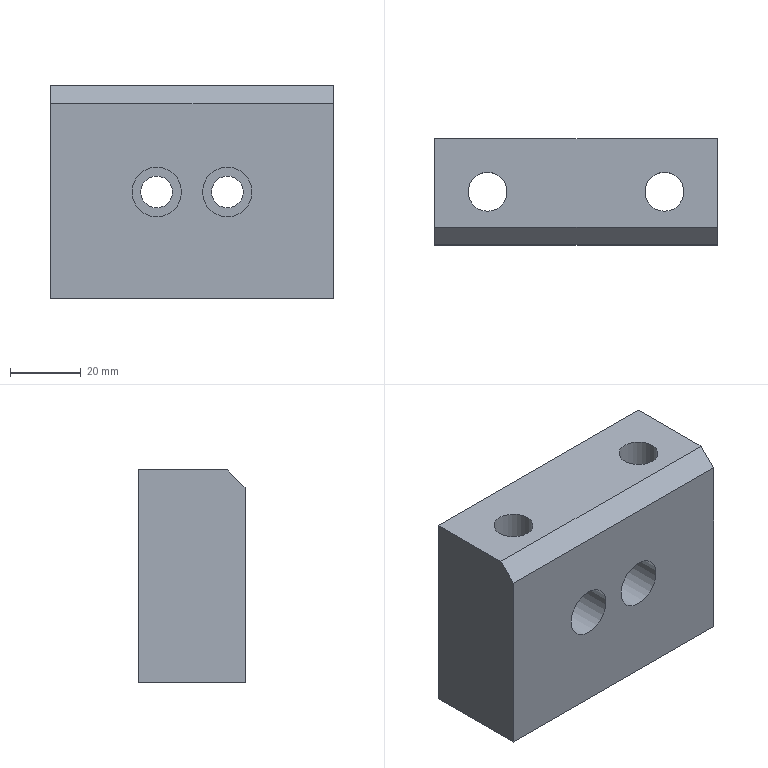Part | NX | features solid 2 | 1 solid | 19 faces | box 80 x 30 x 60 mm | volume 114333 mm3 | plane 11 | cylinder 8 | commonest cylinder face diameters 9 x2 11 x2 14 x2 17.5 x2
STEP:
#1=CARTESIAN_POINT('',(-375.,504.,180.));
#2=VERTEX_POINT('',#1);
#3=CARTESIAN_POINT('',(-375.,529.,180.));
#4=VERTEX_POINT('',#3);
#5=CARTESIAN_POINT('',(-375.,499.,180.));
#6=DIRECTION('',(0.,1.,0.));
#7=VECTOR('',#6,1000.);
#8=LINE('',#5,#7);
#9=EDGE_CURVE('',#2,#4,#8,.T.);
#10=ORIENTED_EDGE('',*,*,#9,.F.);
#11=CARTESIAN_POINT('',(-295.,504.,180.));
#12=VERTEX_POINT('',#11);
#13=CARTESIAN_POINT('',(-325.,504.,180.));
#14=DIRECTION('',(1.,0.,0.));
#15=VECTOR('',#14,1000.);
#16=LINE('',#13,#15);
#17=EDGE_CURVE('',#2,#12,#16,.T.);
#18=ORIENTED_EDGE('',*,*,#17,.T.);
#19=CARTESIAN_POINT('',(-295.,529.,180.));
#20=VERTEX_POINT('',#19);
#21=CARTESIAN_POINT('',(-295.,519.,180.));
#22=DIRECTION('',(0.,1.,0.));
#23=VECTOR('',#22,1000.);
#24=LINE('',#21,#23);
#25=EDGE_CURVE('',#12,#20,#24,.T.);
#26=ORIENTED_EDGE('',*,*,#25,.T.);
#27=CARTESIAN_POINT('',(-325.,529.,180.));
#28=DIRECTION('',(-1.,0.,0.));
#29=VECTOR('',#28,1000.);
#30=LINE('',#27,#29);
#31=EDGE_CURVE('',#20,#4,#30,.T.);
#32=ORIENTED_EDGE('',*,*,#31,.T.);
#33=EDGE_LOOP('',(#10,#18,#26,#32));
#34=FACE_BOUND('',#33,.T.);
#35=CARTESIAN_POINT('',(-310.,519.5,180.));
#36=VERTEX_POINT('',#35);
#37=CARTESIAN_POINT('',(-310.,514.,180.));
#38=DIRECTION('',(0.,0.,-1.));
#39=DIRECTION('',(0.,1.,0.));
#40=AXIS2_PLACEMENT_3D('',#37,#38,#39);
#41=CIRCLE('',#40,5.5);
#42=EDGE_CURVE('',#36,#36,#41,.T.);
#43=ORIENTED_EDGE('',*,*,#42,.T.);
#44=EDGE_LOOP('',(#43));
#45=FACE_BOUND('',#44,.T.);
#46=CARTESIAN_POINT('',(-360.,519.5,180.));
#47=VERTEX_POINT('',#46);
#48=CARTESIAN_POINT('',(-360.,514.,180.));
#49=DIRECTION('',(0.,0.,-1.));
#50=DIRECTION('',(0.,1.,0.));
#51=AXIS2_PLACEMENT_3D('',#48,#49,#50);
#52=CIRCLE('',#51,5.5);
#53=EDGE_CURVE('',#47,#47,#52,.T.);
#54=ORIENTED_EDGE('',*,*,#53,.T.);
#55=EDGE_LOOP('',(#54));
#56=FACE_BOUND('',#55,.T.);
#57=CARTESIAN_POINT('',(-325.,519.,180.));
#58=DIRECTION('',(0.,0.,1.));
#59=DIRECTION('',(-1.,0.,0.));
#60=AXIS2_PLACEMENT_3D('',#57,#58,#59);
#61=PLANE('',#60);
#62=ADVANCED_FACE('',(#34,#45,#56),#61,.T.);
#63=CARTESIAN_POINT('',(-295.,499.,175.));
#64=VERTEX_POINT('',#63);
#65=CARTESIAN_POINT('',(-295.,501.5,177.5));
#66=DIRECTION('',(0.,0.7071,0.7071));
#67=VECTOR('',#66,1000.);
#68=LINE('',#65,#67);
#69=EDGE_CURVE('',#64,#12,#68,.T.);
#70=ORIENTED_EDGE('',*,*,#69,.F.);
#71=CARTESIAN_POINT('',(-295.,499.,120.));
#72=VERTEX_POINT('',#71);
#73=CARTESIAN_POINT('',(-295.,499.,175.));
#74=DIRECTION('',(0.,0.,1.));
#75=VECTOR('',#74,1000.);
#76=LINE('',#73,#75);
#77=EDGE_CURVE('',#64,#72,#76,.F.);
#78=ORIENTED_EDGE('',*,*,#77,.T.);
#79=CARTESIAN_POINT('',(-295.,529.,120.));
#80=VERTEX_POINT('',#79);
#81=CARTESIAN_POINT('',(-295.,662.,120.));
#82=DIRECTION('',(0.,-1.,0.));
#83=VECTOR('',#82,1000.);
#84=LINE('',#81,#83);
#85=EDGE_CURVE('',#72,#80,#84,.F.);
#86=ORIENTED_EDGE('',*,*,#85,.T.);
#87=CARTESIAN_POINT('',(-295.,529.,130.));
#88=DIRECTION('',(0.,0.,1.));
#89=VECTOR('',#88,1000.);
#90=LINE('',#87,#89);
#91=EDGE_CURVE('',#80,#20,#90,.T.);
#92=ORIENTED_EDGE('',*,*,#91,.T.);
#93=ORIENTED_EDGE('',*,*,#25,.F.);
#94=EDGE_LOOP('',(#70,#78,#86,#92,#93));
#95=FACE_BOUND('',#94,.T.);
#96=CARTESIAN_POINT('',(-295.,519.,130.));
#97=DIRECTION('',(1.,0.,0.));
#98=DIRECTION('',(0.,0.,1.));
#99=AXIS2_PLACEMENT_3D('',#96,#97,#98);
#100=PLANE('',#99);
#101=ADVANCED_FACE('',(#95),#100,.T.);
#102=CARTESIAN_POINT('',(-345.,529.,154.5));
#103=VERTEX_POINT('',#102);
#104=CARTESIAN_POINT('',(-345.,529.,150.));
#105=DIRECTION('',(0.,1.,0.));
#106=DIRECTION('',(0.,0.,1.));
#107=AXIS2_PLACEMENT_3D('',#104,#105,#106);
#108=CIRCLE('',#107,4.5);
#109=EDGE_CURVE('',#103,#103,#108,.T.);
#110=ORIENTED_EDGE('',*,*,#109,.F.);
#111=EDGE_LOOP('',(#110));
#112=FACE_BOUND('',#111,.T.);
#113=CARTESIAN_POINT('',(-325.,529.,154.5));
#114=VERTEX_POINT('',#113);
#115=CARTESIAN_POINT('',(-325.,529.,150.));
#116=DIRECTION('',(0.,1.,0.));
#117=DIRECTION('',(0.,0.,1.));
#118=AXIS2_PLACEMENT_3D('',#115,#116,#117);
#119=CIRCLE('',#118,4.5);
#120=EDGE_CURVE('',#114,#114,#119,.T.);
#121=ORIENTED_EDGE('',*,*,#120,.F.);
#122=EDGE_LOOP('',(#121));
#123=FACE_BOUND('',#122,.T.);
#124=CARTESIAN_POINT('',(-375.,529.,120.));
#125=VERTEX_POINT('',#124);
#126=CARTESIAN_POINT('',(-289.,529.,120.));
#127=DIRECTION('',(-1.,0.,0.));
#128=VECTOR('',#127,1000.);
#129=LINE('',#126,#128);
#130=EDGE_CURVE('',#125,#80,#129,.F.);
#131=ORIENTED_EDGE('',*,*,#130,.F.);
#132=CARTESIAN_POINT('',(-375.,529.,175.));
#133=DIRECTION('',(0.,0.,-1.));
#134=VECTOR('',#133,1000.);
#135=LINE('',#132,#134);
#136=EDGE_CURVE('',#4,#125,#135,.T.);
#137=ORIENTED_EDGE('',*,*,#136,.F.);
#138=ORIENTED_EDGE('',*,*,#31,.F.);
#139=ORIENTED_EDGE('',*,*,#91,.F.);
#140=EDGE_LOOP('',(#131,#137,#138,#139));
#141=FACE_BOUND('',#140,.T.);
#142=CARTESIAN_POINT('',(-335.,529.,175.));
#143=DIRECTION('',(0.,-1.,0.));
#144=DIRECTION('',(0.,0.,-1.));
#145=AXIS2_PLACEMENT_3D('',#142,#143,#144);
#146=PLANE('',#145);
#147=ADVANCED_FACE('',(#112,#123,#141),#146,.F.);
#148=CARTESIAN_POINT('',(-345.,499.,143.));
#149=VERTEX_POINT('',#148);
#150=CARTESIAN_POINT('',(-345.,499.,150.));
#151=DIRECTION('',(0.,-1.,0.));
#152=DIRECTION('',(0.,0.,-1.));
#153=AXIS2_PLACEMENT_3D('',#150,#151,#152);
#154=CIRCLE('',#153,7.);
#155=EDGE_CURVE('',#149,#149,#154,.T.);
#156=ORIENTED_EDGE('',*,*,#155,.F.);
#157=EDGE_LOOP('',(#156));
#158=FACE_BOUND('',#157,.T.);
#159=CARTESIAN_POINT('',(-375.,499.,175.));
#160=VERTEX_POINT('',#159);
#161=CARTESIAN_POINT('',(-375.,499.,120.));
#162=VERTEX_POINT('',#161);
#163=CARTESIAN_POINT('',(-375.,499.,175.));
#164=DIRECTION('',(0.,0.,1.));
#165=VECTOR('',#164,1000.);
#166=LINE('',#163,#165);
#167=EDGE_CURVE('',#160,#162,#166,.F.);
#168=ORIENTED_EDGE('',*,*,#167,.T.);
#169=CARTESIAN_POINT('',(-335.,499.,120.));
#170=DIRECTION('',(1.,0.,0.));
#171=VECTOR('',#170,1000.);
#172=LINE('',#169,#171);
#173=EDGE_CURVE('',#162,#72,#172,.T.);
#174=ORIENTED_EDGE('',*,*,#173,.T.);
#175=ORIENTED_EDGE('',*,*,#77,.F.);
#176=CARTESIAN_POINT('',(-335.,499.,175.));
#177=DIRECTION('',(-1.,0.,0.));
#178=VECTOR('',#177,1000.);
#179=LINE('',#176,#178);
#180=EDGE_CURVE('',#160,#64,#179,.F.);
#181=ORIENTED_EDGE('',*,*,#180,.F.);
#182=EDGE_LOOP('',(#168,#174,#175,#181));
#183=FACE_BOUND('',#182,.T.);
#184=CARTESIAN_POINT('',(-325.,499.,143.));
#185=VERTEX_POINT('',#184);
#186=CARTESIAN_POINT('',(-325.,499.,150.));
#187=DIRECTION('',(0.,-1.,0.));
#188=DIRECTION('',(0.,0.,-1.));
#189=AXIS2_PLACEMENT_3D('',#186,#187,#188);
#190=CIRCLE('',#189,7.);
#191=EDGE_CURVE('',#185,#185,#190,.T.);
#192=ORIENTED_EDGE('',*,*,#191,.F.);
#193=EDGE_LOOP('',(#192));
#194=FACE_BOUND('',#193,.T.);
#195=CARTESIAN_POINT('',(-335.,499.,175.));
#196=DIRECTION('',(0.,-1.,0.));
#197=DIRECTION('',(0.,0.,-1.));
#198=AXIS2_PLACEMENT_3D('',#195,#196,#197);
#199=PLANE('',#198);
#200=ADVANCED_FACE('',(#158,#183,#194),#199,.T.);
#201=CARTESIAN_POINT('',(-360.,522.75,120.));
#202=VERTEX_POINT('',#201);
#203=CARTESIAN_POINT('',(-360.,514.,120.));
#204=DIRECTION('',(0.,0.,-1.));
#205=DIRECTION('',(0.,1.,0.));
#206=AXIS2_PLACEMENT_3D('',#203,#204,#205);
#207=CIRCLE('',#206,8.75);
#208=EDGE_CURVE('',#202,#202,#207,.F.);
#209=ORIENTED_EDGE('',*,*,#208,.T.);
#210=EDGE_LOOP('',(#209));
#211=FACE_BOUND('',#210,.T.);
#212=CARTESIAN_POINT('',(-310.,522.75,120.));
#213=VERTEX_POINT('',#212);
#214=CARTESIAN_POINT('',(-310.,514.,120.));
#215=DIRECTION('',(0.,0.,-1.));
#216=DIRECTION('',(0.,1.,0.));
#217=AXIS2_PLACEMENT_3D('',#214,#215,#216);
#218=CIRCLE('',#217,8.75);
#219=EDGE_CURVE('',#213,#213,#218,.F.);
#220=ORIENTED_EDGE('',*,*,#219,.T.);
#221=EDGE_LOOP('',(#220));
#222=FACE_BOUND('',#221,.T.);
#223=CARTESIAN_POINT('',(-375.,662.,120.));
#224=DIRECTION('',(0.,-1.,0.));
#225=VECTOR('',#224,1000.);
#226=LINE('',#223,#225);
#227=EDGE_CURVE('',#162,#125,#226,.F.);
#228=ORIENTED_EDGE('',*,*,#227,.T.);
#229=ORIENTED_EDGE('',*,*,#130,.T.);
#230=ORIENTED_EDGE('',*,*,#85,.F.);
#231=ORIENTED_EDGE('',*,*,#173,.F.);
#232=EDGE_LOOP('',(#228,#229,#230,#231));
#233=FACE_BOUND('',#232,.T.);
#234=CARTESIAN_POINT('',(-289.,662.,120.));
#235=DIRECTION('',(0.,0.,-1.));
#236=DIRECTION('',(1.,0.,0.));
#237=AXIS2_PLACEMENT_3D('',#234,#235,#236);
#238=PLANE('',#237);
#239=ADVANCED_FACE('',(#211,#222,#233),#238,.T.);
#240=ORIENTED_EDGE('',*,*,#9,.T.);
#241=ORIENTED_EDGE('',*,*,#136,.T.);
#242=ORIENTED_EDGE('',*,*,#227,.F.);
#243=ORIENTED_EDGE('',*,*,#167,.F.);
#244=CARTESIAN_POINT('',(-375.,499.,175.));
#245=DIRECTION('',(0.,-0.7071,-0.7071));
#246=VECTOR('',#245,1000.);
#247=LINE('',#244,#246);
#248=EDGE_CURVE('',#2,#160,#247,.T.);
#249=ORIENTED_EDGE('',*,*,#248,.F.);
#250=EDGE_LOOP('',(#240,#241,#242,#243,#249));
#251=FACE_BOUND('',#250,.T.);
#252=CARTESIAN_POINT('',(-375.,499.,175.));
#253=DIRECTION('',(1.,0.,0.));
#254=DIRECTION('',(0.,-0.6428,0.766));
#255=AXIS2_PLACEMENT_3D('',#252,#253,#254);
#256=PLANE('',#255);
#257=ADVANCED_FACE('',(#251),#256,.F.);
#258=CARTESIAN_POINT('',(-310.,508.5,160.));
#259=VERTEX_POINT('',#258);
#260=CARTESIAN_POINT('',(-310.,514.,160.));
#261=DIRECTION('',(0.,0.,1.));
#262=DIRECTION('',(0.,-1.,0.));
#263=AXIS2_PLACEMENT_3D('',#260,#261,#262);
#264=CIRCLE('',#263,5.5);
#265=EDGE_CURVE('',#259,#259,#264,.T.);
#266=ORIENTED_EDGE('',*,*,#265,.F.);
#267=EDGE_LOOP('',(#266));
#268=FACE_BOUND('',#267,.T.);
#269=ORIENTED_EDGE('',*,*,#42,.F.);
#270=EDGE_LOOP('',(#269));
#271=FACE_BOUND('',#270,.T.);
#272=CARTESIAN_POINT('',(-310.,514.,205.));
#273=DIRECTION('',(0.,0.,1.));
#274=DIRECTION('',(0.,-1.,0.));
#275=AXIS2_PLACEMENT_3D('',#272,#273,#274);
#276=CYLINDRICAL_SURFACE('',#275,5.5);
#277=ADVANCED_FACE('',(#268,#271),#276,.F.);
#278=ORIENTED_EDGE('',*,*,#265,.T.);
#279=EDGE_LOOP('',(#278));
#280=FACE_BOUND('',#279,.T.);
#281=CARTESIAN_POINT('',(-310.,505.25,160.));
#282=VERTEX_POINT('',#281);
#283=CARTESIAN_POINT('',(-310.,514.,160.));
#284=DIRECTION('',(0.,0.,1.));
#285=DIRECTION('',(0.,-1.,0.));
#286=AXIS2_PLACEMENT_3D('',#283,#284,#285);
#287=CIRCLE('',#286,8.75);
#288=EDGE_CURVE('',#282,#282,#287,.T.);
#289=ORIENTED_EDGE('',*,*,#288,.F.);
#290=EDGE_LOOP('',(#289));
#291=FACE_BOUND('',#290,.T.);
#292=CARTESIAN_POINT('',(-310.,514.,160.));
#293=DIRECTION('',(0.,0.,1.));
#294=DIRECTION('',(0.,-1.,0.));
#295=AXIS2_PLACEMENT_3D('',#292,#293,#294);
#296=PLANE('',#295);
#297=ADVANCED_FACE('',(#280,#291),#296,.F.);
#298=ORIENTED_EDGE('',*,*,#288,.T.);
#299=EDGE_LOOP('',(#298));
#300=FACE_BOUND('',#299,.T.);
#301=ORIENTED_EDGE('',*,*,#219,.F.);
#302=EDGE_LOOP('',(#301));
#303=FACE_BOUND('',#302,.T.);
#304=CARTESIAN_POINT('',(-310.,514.,125.));
#305=DIRECTION('',(0.,0.,1.));
#306=DIRECTION('',(0.,-1.,0.));
#307=AXIS2_PLACEMENT_3D('',#304,#305,#306);
#308=CYLINDRICAL_SURFACE('',#307,8.75);
#309=ADVANCED_FACE('',(#300,#303),#308,.F.);
#310=CARTESIAN_POINT('',(-325.,509.,154.5));
#311=VERTEX_POINT('',#310);
#312=CARTESIAN_POINT('',(-325.,509.,150.));
#313=DIRECTION('',(0.,1.,0.));
#314=DIRECTION('',(0.,0.,1.));
#315=AXIS2_PLACEMENT_3D('',#312,#313,#314);
#316=CIRCLE('',#315,4.5);
#317=EDGE_CURVE('',#311,#311,#316,.T.);
#318=ORIENTED_EDGE('',*,*,#317,.F.);
#319=EDGE_LOOP('',(#318));
#320=FACE_BOUND('',#319,.T.);
#321=ORIENTED_EDGE('',*,*,#120,.T.);
#322=EDGE_LOOP('',(#321));
#323=FACE_BOUND('',#322,.T.);
#324=CARTESIAN_POINT('',(-325.,529.,150.));
#325=DIRECTION('',(0.,-1.,0.));
#326=DIRECTION('',(0.,0.,-1.));
#327=AXIS2_PLACEMENT_3D('',#324,#325,#326);
#328=CYLINDRICAL_SURFACE('',#327,4.5);
#329=ADVANCED_FACE('',(#320,#323),#328,.F.);
#330=CARTESIAN_POINT('',(-345.,509.,154.5));
#331=VERTEX_POINT('',#330);
#332=CARTESIAN_POINT('',(-345.,509.,150.));
#333=DIRECTION('',(0.,1.,0.));
#334=DIRECTION('',(0.,0.,1.));
#335=AXIS2_PLACEMENT_3D('',#332,#333,#334);
#336=CIRCLE('',#335,4.5);
#337=EDGE_CURVE('',#331,#331,#336,.T.);
#338=ORIENTED_EDGE('',*,*,#337,.F.);
#339=EDGE_LOOP('',(#338));
#340=FACE_BOUND('',#339,.T.);
#341=ORIENTED_EDGE('',*,*,#109,.T.);
#342=EDGE_LOOP('',(#341));
#343=FACE_BOUND('',#342,.T.);
#344=CARTESIAN_POINT('',(-345.,529.,150.));
#345=DIRECTION('',(0.,-1.,0.));
#346=DIRECTION('',(0.,0.,-1.));
#347=AXIS2_PLACEMENT_3D('',#344,#345,#346);
#348=CYLINDRICAL_SURFACE('',#347,4.5);
#349=ADVANCED_FACE('',(#340,#343),#348,.F.);
#350=CARTESIAN_POINT('',(-360.,508.5,160.));
#351=VERTEX_POINT('',#350);
#352=CARTESIAN_POINT('',(-360.,514.,160.));
#353=DIRECTION('',(0.,0.,1.));
#354=DIRECTION('',(0.,-1.,0.));
#355=AXIS2_PLACEMENT_3D('',#352,#353,#354);
#356=CIRCLE('',#355,5.5);
#357=EDGE_CURVE('',#351,#351,#356,.T.);
#358=ORIENTED_EDGE('',*,*,#357,.F.);
#359=EDGE_LOOP('',(#358));
#360=FACE_BOUND('',#359,.T.);
#361=ORIENTED_EDGE('',*,*,#53,.F.);
#362=EDGE_LOOP('',(#361));
#363=FACE_BOUND('',#362,.T.);
#364=CARTESIAN_POINT('',(-360.,514.,205.));
#365=DIRECTION('',(0.,0.,1.));
#366=DIRECTION('',(0.,-1.,0.));
#367=AXIS2_PLACEMENT_3D('',#364,#365,#366);
#368=CYLINDRICAL_SURFACE('',#367,5.5);
#369=ADVANCED_FACE('',(#360,#363),#368,.F.);
#370=ORIENTED_EDGE('',*,*,#357,.T.);
#371=EDGE_LOOP('',(#370));
#372=FACE_BOUND('',#371,.T.);
#373=CARTESIAN_POINT('',(-360.,505.25,160.));
#374=VERTEX_POINT('',#373);
#375=CARTESIAN_POINT('',(-360.,514.,160.));
#376=DIRECTION('',(0.,0.,1.));
#377=DIRECTION('',(0.,-1.,0.));
#378=AXIS2_PLACEMENT_3D('',#375,#376,#377);
#379=CIRCLE('',#378,8.75);
#380=EDGE_CURVE('',#374,#374,#379,.T.);
#381=ORIENTED_EDGE('',*,*,#380,.F.);
#382=EDGE_LOOP('',(#381));
#383=FACE_BOUND('',#382,.T.);
#384=CARTESIAN_POINT('',(-360.,514.,160.));
#385=DIRECTION('',(0.,0.,1.));
#386=DIRECTION('',(0.,-1.,0.));
#387=AXIS2_PLACEMENT_3D('',#384,#385,#386);
#388=PLANE('',#387);
#389=ADVANCED_FACE('',(#372,#383),#388,.F.);
#390=ORIENTED_EDGE('',*,*,#380,.T.);
#391=EDGE_LOOP('',(#390));
#392=FACE_BOUND('',#391,.T.);
#393=ORIENTED_EDGE('',*,*,#208,.F.);
#394=EDGE_LOOP('',(#393));
#395=FACE_BOUND('',#394,.T.);
#396=CARTESIAN_POINT('',(-360.,514.,125.));
#397=DIRECTION('',(0.,0.,1.));
#398=DIRECTION('',(0.,-1.,0.));
#399=AXIS2_PLACEMENT_3D('',#396,#397,#398);
#400=CYLINDRICAL_SURFACE('',#399,8.75);
#401=ADVANCED_FACE('',(#392,#395),#400,.F.);
#402=CARTESIAN_POINT('',(-345.,509.,157.));
#403=VERTEX_POINT('',#402);
#404=CARTESIAN_POINT('',(-345.,509.,150.));
#405=DIRECTION('',(0.,1.,0.));
#406=DIRECTION('',(0.,0.,1.));
#407=AXIS2_PLACEMENT_3D('',#404,#405,#406);
#408=CIRCLE('',#407,7.);
#409=EDGE_CURVE('',#403,#403,#408,.T.);
#410=ORIENTED_EDGE('',*,*,#409,.T.);
#411=EDGE_LOOP('',(#410));
#412=FACE_BOUND('',#411,.T.);
#413=ORIENTED_EDGE('',*,*,#155,.T.);
#414=EDGE_LOOP('',(#413));
#415=FACE_BOUND('',#414,.T.);
#416=CARTESIAN_POINT('',(-345.,514.,150.));
#417=DIRECTION('',(0.,-1.,0.));
#418=DIRECTION('',(0.,0.,-1.));
#419=AXIS2_PLACEMENT_3D('',#416,#417,#418);
#420=CYLINDRICAL_SURFACE('',#419,7.);
#421=ADVANCED_FACE('',(#412,#415),#420,.F.);
#422=ORIENTED_EDGE('',*,*,#337,.T.);
#423=EDGE_LOOP('',(#422));
#424=FACE_BOUND('',#423,.T.);
#425=ORIENTED_EDGE('',*,*,#409,.F.);
#426=EDGE_LOOP('',(#425));
#427=FACE_BOUND('',#426,.T.);
#428=CARTESIAN_POINT('',(-345.,509.,150.));
#429=DIRECTION('',(0.,1.,0.));
#430=DIRECTION('',(0.,0.,1.));
#431=AXIS2_PLACEMENT_3D('',#428,#429,#430);
#432=PLANE('',#431);
#433=ADVANCED_FACE('',(#424,#427),#432,.F.);
#434=CARTESIAN_POINT('',(-325.,509.,157.));
#435=VERTEX_POINT('',#434);
#436=CARTESIAN_POINT('',(-325.,509.,150.));
#437=DIRECTION('',(0.,1.,0.));
#438=DIRECTION('',(0.,0.,1.));
#439=AXIS2_PLACEMENT_3D('',#436,#437,#438);
#440=CIRCLE('',#439,7.);
#441=EDGE_CURVE('',#435,#435,#440,.T.);
#442=ORIENTED_EDGE('',*,*,#441,.T.);
#443=EDGE_LOOP('',(#442));
#444=FACE_BOUND('',#443,.T.);
#445=ORIENTED_EDGE('',*,*,#191,.T.);
#446=EDGE_LOOP('',(#445));
#447=FACE_BOUND('',#446,.T.);
#448=CARTESIAN_POINT('',(-325.,514.,150.));
#449=DIRECTION('',(0.,-1.,0.));
#450=DIRECTION('',(0.,0.,-1.));
#451=AXIS2_PLACEMENT_3D('',#448,#449,#450);
#452=CYLINDRICAL_SURFACE('',#451,7.);
#453=ADVANCED_FACE('',(#444,#447),#452,.F.);
#454=ORIENTED_EDGE('',*,*,#317,.T.);
#455=EDGE_LOOP('',(#454));
#456=FACE_BOUND('',#455,.T.);
#457=ORIENTED_EDGE('',*,*,#441,.F.);
#458=EDGE_LOOP('',(#457));
#459=FACE_BOUND('',#458,.T.);
#460=CARTESIAN_POINT('',(-325.,509.,150.));
#461=DIRECTION('',(0.,1.,0.));
#462=DIRECTION('',(0.,0.,1.));
#463=AXIS2_PLACEMENT_3D('',#460,#461,#462);
#464=PLANE('',#463);
#465=ADVANCED_FACE('',(#456,#459),#464,.F.);
#466=ORIENTED_EDGE('',*,*,#248,.T.);
#467=ORIENTED_EDGE('',*,*,#180,.T.);
#468=ORIENTED_EDGE('',*,*,#69,.T.);
#469=ORIENTED_EDGE('',*,*,#17,.F.);
#470=EDGE_LOOP('',(#466,#467,#468,#469));
#471=FACE_BOUND('',#470,.T.);
#472=CARTESIAN_POINT('',(-335.,499.,175.));
#473=DIRECTION('',(0.,-0.7071,0.7071));
#474=DIRECTION('',(0.,0.7071,0.7071));
#475=AXIS2_PLACEMENT_3D('',#472,#473,#474);
#476=PLANE('',#475);
#477=ADVANCED_FACE('',(#471),#476,.T.);
#478=CLOSED_SHELL('',(#62,#101,#147,#200,#239,#257,#277,#297,#309,#329,#349,#369,#389,#401,#421,#433,#453,#465,#477));
#479=MANIFOLD_SOLID_BREP('',#478);
#480=(LENGTH_UNIT()NAMED_UNIT(*)SI_UNIT(.MILLI.,.METRE.));
#481=UNCERTAINTY_MEASURE_WITH_UNIT(LENGTH_MEASURE(0.00001),#480,'','');
#482=(NAMED_UNIT(*)PLANE_ANGLE_UNIT()SI_UNIT($,.RADIAN.));
#483=(NAMED_UNIT(*)SI_UNIT($,.STERADIAN.)SOLID_ANGLE_UNIT());
#484=(GEOMETRIC_REPRESENTATION_CONTEXT(3)GLOBAL_UNCERTAINTY_ASSIGNED_CONTEXT((#481))GLOBAL_UNIT_ASSIGNED_CONTEXT((#480,#482,#483))REPRESENTATION_CONTEXT('',''));
#485=ADVANCED_BREP_SHAPE_REPRESENTATION('',(#479),#484);